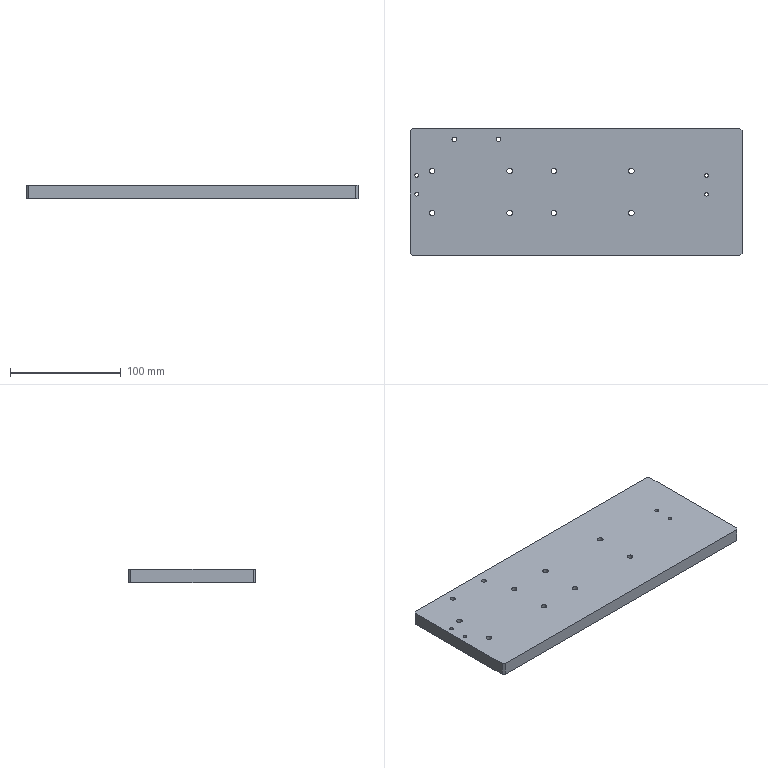Part | SolidWorks | features HoleWzd 3, Chamfer 1, Extrusion 1 | 1 solid | 38 faces | box 300 x 115 x 12 mm | volume 411276 mm3 | cylinder 28 | plane 10 | commonest cylinder face diameters 5 x16 3.3 x8 4.2 x4
STEP:
#1=CARTESIAN_POINT('',(-107.9,47.5,12.));
#2=VERTEX_POINT('',#1);
#3=CARTESIAN_POINT('',(-112.1,47.5,12.));
#4=VERTEX_POINT('',#3);
#5=CARTESIAN_POINT('',(-110.,47.5,12.));
#6=DIRECTION('',(0.,0.,-1.));
#7=DIRECTION('',(-1.,0.,0.));
#8=AXIS2_PLACEMENT_3D('',#5,#6,#7);
#9=CIRCLE('',#8,2.1);
#10=EDGE_CURVE('',#2,#4,#9,.T.);
#11=ORIENTED_EDGE('',*,*,#10,.F.);
#12=CARTESIAN_POINT('',(-107.9,47.5,0.));
#13=VERTEX_POINT('',#12);
#14=CARTESIAN_POINT('',(-107.9,47.5,0.));
#15=DIRECTION('',(0.,0.,-1.));
#16=VECTOR('',#15,1000.);
#17=LINE('',#14,#16);
#18=EDGE_CURVE('',#2,#13,#17,.T.);
#19=ORIENTED_EDGE('',*,*,#18,.T.);
#20=CARTESIAN_POINT('',(-112.1,47.5,0.));
#21=VERTEX_POINT('',#20);
#22=CARTESIAN_POINT('',(-110.,47.5,0.));
#23=DIRECTION('',(0.,0.,-1.));
#24=DIRECTION('',(-1.,0.,0.));
#25=AXIS2_PLACEMENT_3D('',#22,#23,#24);
#26=CIRCLE('',#25,2.1);
#27=EDGE_CURVE('',#13,#21,#26,.T.);
#28=ORIENTED_EDGE('',*,*,#27,.T.);
#29=CARTESIAN_POINT('',(-112.1,47.5,0.));
#30=DIRECTION('',(0.,0.,-1.));
#31=VECTOR('',#30,1000.);
#32=LINE('',#29,#31);
#33=EDGE_CURVE('',#4,#21,#32,.T.);
#34=ORIENTED_EDGE('',*,*,#33,.F.);
#35=EDGE_LOOP('',(#11,#19,#28,#34));
#36=FACE_OUTER_BOUND('',#35,.T.);
#37=CARTESIAN_POINT('',(-110.,47.5,0.));
#38=DIRECTION('',(0.,0.,-1.));
#39=DIRECTION('',(-1.,0.,0.));
#40=AXIS2_PLACEMENT_3D('',#37,#38,#39);
#41=CYLINDRICAL_SURFACE('',#40,2.1);
#42=ADVANCED_FACE('',(#36),#41,.F.);
#43=CARTESIAN_POINT('',(-67.9,47.5,12.));
#44=VERTEX_POINT('',#43);
#45=CARTESIAN_POINT('',(-72.1,47.5,12.));
#46=VERTEX_POINT('',#45);
#47=CARTESIAN_POINT('',(-70.,47.5,12.));
#48=DIRECTION('',(0.,0.,-1.));
#49=DIRECTION('',(-1.,0.,0.));
#50=AXIS2_PLACEMENT_3D('',#47,#48,#49);
#51=CIRCLE('',#50,2.1);
#52=EDGE_CURVE('',#44,#46,#51,.T.);
#53=ORIENTED_EDGE('',*,*,#52,.F.);
#54=CARTESIAN_POINT('',(-67.9,47.5,0.));
#55=VERTEX_POINT('',#54);
#56=CARTESIAN_POINT('',(-67.9,47.5,0.));
#57=DIRECTION('',(0.,0.,-1.));
#58=VECTOR('',#57,1000.);
#59=LINE('',#56,#58);
#60=EDGE_CURVE('',#44,#55,#59,.T.);
#61=ORIENTED_EDGE('',*,*,#60,.T.);
#62=CARTESIAN_POINT('',(-72.1,47.5,0.));
#63=VERTEX_POINT('',#62);
#64=CARTESIAN_POINT('',(-70.,47.5,0.));
#65=DIRECTION('',(0.,0.,-1.));
#66=DIRECTION('',(-1.,0.,0.));
#67=AXIS2_PLACEMENT_3D('',#64,#65,#66);
#68=CIRCLE('',#67,2.1);
#69=EDGE_CURVE('',#55,#63,#68,.T.);
#70=ORIENTED_EDGE('',*,*,#69,.T.);
#71=CARTESIAN_POINT('',(-72.1,47.5,0.));
#72=DIRECTION('',(0.,0.,-1.));
#73=VECTOR('',#72,1000.);
#74=LINE('',#71,#73);
#75=EDGE_CURVE('',#46,#63,#74,.T.);
#76=ORIENTED_EDGE('',*,*,#75,.F.);
#77=EDGE_LOOP('',(#53,#61,#70,#76));
#78=FACE_OUTER_BOUND('',#77,.T.);
#79=CARTESIAN_POINT('',(-70.,47.5,0.));
#80=DIRECTION('',(0.,0.,-1.));
#81=DIRECTION('',(-1.,0.,0.));
#82=AXIS2_PLACEMENT_3D('',#79,#80,#81);
#83=CYLINDRICAL_SURFACE('',#82,2.1);
#84=ADVANCED_FACE('',(#78),#83,.F.);
#85=CARTESIAN_POINT('',(-145.65,15.,0.));
#86=VERTEX_POINT('',#85);
#87=CARTESIAN_POINT('',(-142.35,15.,0.));
#88=VERTEX_POINT('',#87);
#89=CARTESIAN_POINT('',(-144.,15.,0.));
#90=DIRECTION('',(0.,0.,1.));
#91=DIRECTION('',(1.,0.,0.));
#92=AXIS2_PLACEMENT_3D('',#89,#90,#91);
#93=CIRCLE('',#92,1.65);
#94=EDGE_CURVE('',#86,#88,#93,.T.);
#95=ORIENTED_EDGE('',*,*,#94,.F.);
#96=CARTESIAN_POINT('',(-145.65,15.,12.));
#97=VERTEX_POINT('',#96);
#98=CARTESIAN_POINT('',(-145.65,15.,12.));
#99=DIRECTION('',(0.,0.,1.));
#100=VECTOR('',#99,1000.);
#101=LINE('',#98,#100);
#102=EDGE_CURVE('',#86,#97,#101,.T.);
#103=ORIENTED_EDGE('',*,*,#102,.T.);
#104=CARTESIAN_POINT('',(-142.35,15.,12.));
#105=VERTEX_POINT('',#104);
#106=CARTESIAN_POINT('',(-144.,15.,12.));
#107=DIRECTION('',(0.,0.,1.));
#108=DIRECTION('',(1.,0.,0.));
#109=AXIS2_PLACEMENT_3D('',#106,#107,#108);
#110=CIRCLE('',#109,1.65);
#111=EDGE_CURVE('',#97,#105,#110,.T.);
#112=ORIENTED_EDGE('',*,*,#111,.T.);
#113=CARTESIAN_POINT('',(-142.35,15.,12.));
#114=DIRECTION('',(0.,0.,1.));
#115=VECTOR('',#114,1000.);
#116=LINE('',#113,#115);
#117=EDGE_CURVE('',#88,#105,#116,.T.);
#118=ORIENTED_EDGE('',*,*,#117,.F.);
#119=EDGE_LOOP('',(#95,#103,#112,#118));
#120=FACE_OUTER_BOUND('',#119,.T.);
#121=CARTESIAN_POINT('',(-144.,15.,12.));
#122=DIRECTION('',(0.,0.,1.));
#123=DIRECTION('',(1.,0.,0.));
#124=AXIS2_PLACEMENT_3D('',#121,#122,#123);
#125=CYLINDRICAL_SURFACE('',#124,1.65);
#126=ADVANCED_FACE('',(#120),#125,.F.);
#127=CARTESIAN_POINT('',(-145.65,-2.,0.));
#128=VERTEX_POINT('',#127);
#129=CARTESIAN_POINT('',(-142.35,-2.,0.));
#130=VERTEX_POINT('',#129);
#131=CARTESIAN_POINT('',(-144.,-2.,0.));
#132=DIRECTION('',(0.,0.,1.));
#133=DIRECTION('',(1.,0.,0.));
#134=AXIS2_PLACEMENT_3D('',#131,#132,#133);
#135=CIRCLE('',#134,1.65);
#136=EDGE_CURVE('',#128,#130,#135,.T.);
#137=ORIENTED_EDGE('',*,*,#136,.F.);
#138=CARTESIAN_POINT('',(-145.65,-2.,12.));
#139=VERTEX_POINT('',#138);
#140=CARTESIAN_POINT('',(-145.65,-2.,12.));
#141=DIRECTION('',(0.,0.,1.));
#142=VECTOR('',#141,1000.);
#143=LINE('',#140,#142);
#144=EDGE_CURVE('',#128,#139,#143,.T.);
#145=ORIENTED_EDGE('',*,*,#144,.T.);
#146=CARTESIAN_POINT('',(-142.35,-2.,12.));
#147=VERTEX_POINT('',#146);
#148=CARTESIAN_POINT('',(-144.,-2.,12.));
#149=DIRECTION('',(0.,0.,1.));
#150=DIRECTION('',(1.,0.,0.));
#151=AXIS2_PLACEMENT_3D('',#148,#149,#150);
#152=CIRCLE('',#151,1.65);
#153=EDGE_CURVE('',#139,#147,#152,.T.);
#154=ORIENTED_EDGE('',*,*,#153,.T.);
#155=CARTESIAN_POINT('',(-142.35,-2.,12.));
#156=DIRECTION('',(0.,0.,1.));
#157=VECTOR('',#156,1000.);
#158=LINE('',#155,#157);
#159=EDGE_CURVE('',#130,#147,#158,.T.);
#160=ORIENTED_EDGE('',*,*,#159,.F.);
#161=EDGE_LOOP('',(#137,#145,#154,#160));
#162=FACE_OUTER_BOUND('',#161,.T.);
#163=CARTESIAN_POINT('',(-144.,-2.,12.));
#164=DIRECTION('',(0.,0.,1.));
#165=DIRECTION('',(1.,0.,0.));
#166=AXIS2_PLACEMENT_3D('',#163,#164,#165);
#167=CYLINDRICAL_SURFACE('',#166,1.65);
#168=ADVANCED_FACE('',(#162),#167,.F.);
#169=CARTESIAN_POINT('',(116.35,15.,0.));
#170=VERTEX_POINT('',#169);
#171=CARTESIAN_POINT('',(119.65,15.,0.));
#172=VERTEX_POINT('',#171);
#173=CARTESIAN_POINT('',(118.,15.,0.));
#174=DIRECTION('',(0.,0.,1.));
#175=DIRECTION('',(1.,0.,0.));
#176=AXIS2_PLACEMENT_3D('',#173,#174,#175);
#177=CIRCLE('',#176,1.65);
#178=EDGE_CURVE('',#170,#172,#177,.T.);
#179=ORIENTED_EDGE('',*,*,#178,.F.);
#180=CARTESIAN_POINT('',(116.35,15.,12.));
#181=VERTEX_POINT('',#180);
#182=CARTESIAN_POINT('',(116.35,15.,12.));
#183=DIRECTION('',(0.,0.,1.));
#184=VECTOR('',#183,1000.);
#185=LINE('',#182,#184);
#186=EDGE_CURVE('',#170,#181,#185,.T.);
#187=ORIENTED_EDGE('',*,*,#186,.T.);
#188=CARTESIAN_POINT('',(119.65,15.,12.));
#189=VERTEX_POINT('',#188);
#190=CARTESIAN_POINT('',(118.,15.,12.));
#191=DIRECTION('',(0.,0.,1.));
#192=DIRECTION('',(1.,0.,0.));
#193=AXIS2_PLACEMENT_3D('',#190,#191,#192);
#194=CIRCLE('',#193,1.65);
#195=EDGE_CURVE('',#181,#189,#194,.T.);
#196=ORIENTED_EDGE('',*,*,#195,.T.);
#197=CARTESIAN_POINT('',(119.65,15.,12.));
#198=DIRECTION('',(0.,0.,1.));
#199=VECTOR('',#198,1000.);
#200=LINE('',#197,#199);
#201=EDGE_CURVE('',#172,#189,#200,.T.);
#202=ORIENTED_EDGE('',*,*,#201,.F.);
#203=EDGE_LOOP('',(#179,#187,#196,#202));
#204=FACE_OUTER_BOUND('',#203,.T.);
#205=CARTESIAN_POINT('',(118.,15.,12.));
#206=DIRECTION('',(0.,0.,1.));
#207=DIRECTION('',(1.,0.,0.));
#208=AXIS2_PLACEMENT_3D('',#205,#206,#207);
#209=CYLINDRICAL_SURFACE('',#208,1.65);
#210=ADVANCED_FACE('',(#204),#209,.F.);
#211=CARTESIAN_POINT('',(116.35,-2.,0.));
#212=VERTEX_POINT('',#211);
#213=CARTESIAN_POINT('',(119.65,-2.,0.));
#214=VERTEX_POINT('',#213);
#215=CARTESIAN_POINT('',(118.,-2.,0.));
#216=DIRECTION('',(0.,0.,1.));
#217=DIRECTION('',(1.,0.,0.));
#218=AXIS2_PLACEMENT_3D('',#215,#216,#217);
#219=CIRCLE('',#218,1.65);
#220=EDGE_CURVE('',#212,#214,#219,.T.);
#221=ORIENTED_EDGE('',*,*,#220,.F.);
#222=CARTESIAN_POINT('',(116.35,-2.,12.));
#223=VERTEX_POINT('',#222);
#224=CARTESIAN_POINT('',(116.35,-2.,12.));
#225=DIRECTION('',(0.,0.,1.));
#226=VECTOR('',#225,1000.);
#227=LINE('',#224,#226);
#228=EDGE_CURVE('',#212,#223,#227,.T.);
#229=ORIENTED_EDGE('',*,*,#228,.T.);
#230=CARTESIAN_POINT('',(119.65,-2.,12.));
#231=VERTEX_POINT('',#230);
#232=CARTESIAN_POINT('',(118.,-2.,12.));
#233=DIRECTION('',(0.,0.,1.));
#234=DIRECTION('',(1.,0.,0.));
#235=AXIS2_PLACEMENT_3D('',#232,#233,#234);
#236=CIRCLE('',#235,1.65);
#237=EDGE_CURVE('',#223,#231,#236,.T.);
#238=ORIENTED_EDGE('',*,*,#237,.T.);
#239=CARTESIAN_POINT('',(119.65,-2.,12.));
#240=DIRECTION('',(0.,0.,1.));
#241=VECTOR('',#240,1000.);
#242=LINE('',#239,#241);
#243=EDGE_CURVE('',#214,#231,#242,.T.);
#244=ORIENTED_EDGE('',*,*,#243,.F.);
#245=EDGE_LOOP('',(#221,#229,#238,#244));
#246=FACE_OUTER_BOUND('',#245,.T.);
#247=CARTESIAN_POINT('',(118.,-2.,12.));
#248=DIRECTION('',(0.,0.,1.));
#249=DIRECTION('',(1.,0.,0.));
#250=AXIS2_PLACEMENT_3D('',#247,#248,#249);
#251=CYLINDRICAL_SURFACE('',#250,1.65);
#252=ADVANCED_FACE('',(#246),#251,.F.);
#253=CARTESIAN_POINT('',(-127.5,19.,12.));
#254=VERTEX_POINT('',#253);
#255=CARTESIAN_POINT('',(-132.5,19.,12.));
#256=VERTEX_POINT('',#255);
#257=CARTESIAN_POINT('',(-130.,19.,12.));
#258=DIRECTION('',(0.,0.,-1.));
#259=DIRECTION('',(-1.,0.,0.));
#260=AXIS2_PLACEMENT_3D('',#257,#258,#259);
#261=CIRCLE('',#260,2.5);
#262=EDGE_CURVE('',#254,#256,#261,.T.);
#263=ORIENTED_EDGE('',*,*,#262,.F.);
#264=CARTESIAN_POINT('',(-127.5,19.,0.));
#265=VERTEX_POINT('',#264);
#266=CARTESIAN_POINT('',(-127.5,19.,0.));
#267=DIRECTION('',(0.,0.,-1.));
#268=VECTOR('',#267,1000.);
#269=LINE('',#266,#268);
#270=EDGE_CURVE('',#254,#265,#269,.T.);
#271=ORIENTED_EDGE('',*,*,#270,.T.);
#272=CARTESIAN_POINT('',(-132.5,19.,0.));
#273=VERTEX_POINT('',#272);
#274=CARTESIAN_POINT('',(-130.,19.,0.));
#275=DIRECTION('',(0.,0.,-1.));
#276=DIRECTION('',(-1.,0.,0.));
#277=AXIS2_PLACEMENT_3D('',#274,#275,#276);
#278=CIRCLE('',#277,2.5);
#279=EDGE_CURVE('',#265,#273,#278,.T.);
#280=ORIENTED_EDGE('',*,*,#279,.T.);
#281=CARTESIAN_POINT('',(-132.5,19.,0.));
#282=DIRECTION('',(0.,0.,-1.));
#283=VECTOR('',#282,1000.);
#284=LINE('',#281,#283);
#285=EDGE_CURVE('',#256,#273,#284,.T.);
#286=ORIENTED_EDGE('',*,*,#285,.F.);
#287=EDGE_LOOP('',(#263,#271,#280,#286));
#288=FACE_OUTER_BOUND('',#287,.T.);
#289=CARTESIAN_POINT('',(-130.,19.,0.));
#290=DIRECTION('',(0.,0.,-1.));
#291=DIRECTION('',(-1.,0.,0.));
#292=AXIS2_PLACEMENT_3D('',#289,#290,#291);
#293=CYLINDRICAL_SURFACE('',#292,2.5);
#294=ADVANCED_FACE('',(#288),#293,.F.);
#295=CARTESIAN_POINT('',(-57.5,-19.,12.));
#296=VERTEX_POINT('',#295);
#297=CARTESIAN_POINT('',(-62.5,-19.,12.));
#298=VERTEX_POINT('',#297);
#299=CARTESIAN_POINT('',(-60.,-19.,12.));
#300=DIRECTION('',(0.,0.,-1.));
#301=DIRECTION('',(-1.,0.,0.));
#302=AXIS2_PLACEMENT_3D('',#299,#300,#301);
#303=CIRCLE('',#302,2.5);
#304=EDGE_CURVE('',#296,#298,#303,.T.);
#305=ORIENTED_EDGE('',*,*,#304,.F.);
#306=CARTESIAN_POINT('',(-57.5,-19.,0.));
#307=VERTEX_POINT('',#306);
#308=CARTESIAN_POINT('',(-57.5,-19.,0.));
#309=DIRECTION('',(0.,0.,-1.));
#310=VECTOR('',#309,1000.);
#311=LINE('',#308,#310);
#312=EDGE_CURVE('',#296,#307,#311,.T.);
#313=ORIENTED_EDGE('',*,*,#312,.T.);
#314=CARTESIAN_POINT('',(-62.5,-19.,0.));
#315=VERTEX_POINT('',#314);
#316=CARTESIAN_POINT('',(-60.,-19.,0.));
#317=DIRECTION('',(0.,0.,-1.));
#318=DIRECTION('',(-1.,0.,0.));
#319=AXIS2_PLACEMENT_3D('',#316,#317,#318);
#320=CIRCLE('',#319,2.5);
#321=EDGE_CURVE('',#307,#315,#320,.T.);
#322=ORIENTED_EDGE('',*,*,#321,.T.);
#323=CARTESIAN_POINT('',(-62.5,-19.,0.));
#324=DIRECTION('',(0.,0.,-1.));
#325=VECTOR('',#324,1000.);
#326=LINE('',#323,#325);
#327=EDGE_CURVE('',#298,#315,#326,.T.);
#328=ORIENTED_EDGE('',*,*,#327,.F.);
#329=EDGE_LOOP('',(#305,#313,#322,#328));
#330=FACE_OUTER_BOUND('',#329,.T.);
#331=CARTESIAN_POINT('',(-60.,-19.,0.));
#332=DIRECTION('',(0.,0.,-1.));
#333=DIRECTION('',(-1.,0.,0.));
#334=AXIS2_PLACEMENT_3D('',#331,#332,#333);
#335=CYLINDRICAL_SURFACE('',#334,2.5);
#336=ADVANCED_FACE('',(#330),#335,.F.);
#337=CARTESIAN_POINT('',(-57.5,19.,12.));
#338=VERTEX_POINT('',#337);
#339=CARTESIAN_POINT('',(-62.5,19.,12.));
#340=VERTEX_POINT('',#339);
#341=CARTESIAN_POINT('',(-60.,19.,12.));
#342=DIRECTION('',(0.,0.,-1.));
#343=DIRECTION('',(-1.,0.,0.));
#344=AXIS2_PLACEMENT_3D('',#341,#342,#343);
#345=CIRCLE('',#344,2.5);
#346=EDGE_CURVE('',#338,#340,#345,.T.);
#347=ORIENTED_EDGE('',*,*,#346,.F.);
#348=CARTESIAN_POINT('',(-57.5,19.,0.));
#349=VERTEX_POINT('',#348);
#350=CARTESIAN_POINT('',(-57.5,19.,0.));
#351=DIRECTION('',(0.,0.,-1.));
#352=VECTOR('',#351,1000.);
#353=LINE('',#350,#352);
#354=EDGE_CURVE('',#338,#349,#353,.T.);
#355=ORIENTED_EDGE('',*,*,#354,.T.);
#356=CARTESIAN_POINT('',(-62.5,19.,0.));
#357=VERTEX_POINT('',#356);
#358=CARTESIAN_POINT('',(-60.,19.,0.));
#359=DIRECTION('',(0.,0.,-1.));
#360=DIRECTION('',(-1.,0.,0.));
#361=AXIS2_PLACEMENT_3D('',#358,#359,#360);
#362=CIRCLE('',#361,2.5);
#363=EDGE_CURVE('',#349,#357,#362,.T.);
#364=ORIENTED_EDGE('',*,*,#363,.T.);
#365=CARTESIAN_POINT('',(-62.5,19.,0.));
#366=DIRECTION('',(0.,0.,-1.));
#367=VECTOR('',#366,1000.);
#368=LINE('',#365,#367);
#369=EDGE_CURVE('',#340,#357,#368,.T.);
#370=ORIENTED_EDGE('',*,*,#369,.F.);
#371=EDGE_LOOP('',(#347,#355,#364,#370));
#372=FACE_OUTER_BOUND('',#371,.T.);
#373=CARTESIAN_POINT('',(-60.,19.,0.));
#374=DIRECTION('',(0.,0.,-1.));
#375=DIRECTION('',(-1.,0.,0.));
#376=AXIS2_PLACEMENT_3D('',#373,#374,#375);
#377=CYLINDRICAL_SURFACE('',#376,2.5);
#378=ADVANCED_FACE('',(#372),#377,.F.);
#379=CARTESIAN_POINT('',(-127.5,-19.,12.));
#380=VERTEX_POINT('',#379);
#381=CARTESIAN_POINT('',(-132.5,-19.,12.));
#382=VERTEX_POINT('',#381);
#383=CARTESIAN_POINT('',(-130.,-19.,12.));
#384=DIRECTION('',(0.,0.,-1.));
#385=DIRECTION('',(-1.,0.,0.));
#386=AXIS2_PLACEMENT_3D('',#383,#384,#385);
#387=CIRCLE('',#386,2.5);
#388=EDGE_CURVE('',#380,#382,#387,.T.);
#389=ORIENTED_EDGE('',*,*,#388,.F.);
#390=CARTESIAN_POINT('',(-127.5,-19.,0.));
#391=VERTEX_POINT('',#390);
#392=CARTESIAN_POINT('',(-127.5,-19.,0.));
#393=DIRECTION('',(0.,0.,-1.));
#394=VECTOR('',#393,1000.);
#395=LINE('',#392,#394);
#396=EDGE_CURVE('',#380,#391,#395,.T.);
#397=ORIENTED_EDGE('',*,*,#396,.T.);
#398=CARTESIAN_POINT('',(-132.5,-19.,0.));
#399=VERTEX_POINT('',#398);
#400=CARTESIAN_POINT('',(-130.,-19.,0.));
#401=DIRECTION('',(0.,0.,-1.));
#402=DIRECTION('',(-1.,0.,0.));
#403=AXIS2_PLACEMENT_3D('',#400,#401,#402);
#404=CIRCLE('',#403,2.5);
#405=EDGE_CURVE('',#391,#399,#404,.T.);
#406=ORIENTED_EDGE('',*,*,#405,.T.);
#407=CARTESIAN_POINT('',(-132.5,-19.,0.));
#408=DIRECTION('',(0.,0.,-1.));
#409=VECTOR('',#408,1000.);
#410=LINE('',#407,#409);
#411=EDGE_CURVE('',#382,#399,#410,.T.);
#412=ORIENTED_EDGE('',*,*,#411,.F.);
#413=EDGE_LOOP('',(#389,#397,#406,#412));
#414=FACE_OUTER_BOUND('',#413,.T.);
#415=CARTESIAN_POINT('',(-130.,-19.,0.));
#416=DIRECTION('',(0.,0.,-1.));
#417=DIRECTION('',(-1.,0.,0.));
#418=AXIS2_PLACEMENT_3D('',#415,#416,#417);
#419=CYLINDRICAL_SURFACE('',#418,2.5);
#420=ADVANCED_FACE('',(#414),#419,.F.);
#421=CARTESIAN_POINT('',(-17.5,19.,12.));
#422=VERTEX_POINT('',#421);
#423=CARTESIAN_POINT('',(-22.5,19.,12.));
#424=VERTEX_POINT('',#423);
#425=CARTESIAN_POINT('',(-20.,19.,12.));
#426=DIRECTION('',(0.,0.,-1.));
#427=DIRECTION('',(-1.,0.,0.));
#428=AXIS2_PLACEMENT_3D('',#425,#426,#427);
#429=CIRCLE('',#428,2.5);
#430=EDGE_CURVE('',#422,#424,#429,.T.);
#431=ORIENTED_EDGE('',*,*,#430,.F.);
#432=CARTESIAN_POINT('',(-17.5,19.,0.));
#433=VERTEX_POINT('',#432);
#434=CARTESIAN_POINT('',(-17.5,19.,0.));
#435=DIRECTION('',(0.,0.,-1.));
#436=VECTOR('',#435,1000.);
#437=LINE('',#434,#436);
#438=EDGE_CURVE('',#422,#433,#437,.T.);
#439=ORIENTED_EDGE('',*,*,#438,.T.);
#440=CARTESIAN_POINT('',(-22.5,19.,0.));
#441=VERTEX_POINT('',#440);
#442=CARTESIAN_POINT('',(-20.,19.,0.));
#443=DIRECTION('',(0.,0.,-1.));
#444=DIRECTION('',(-1.,0.,0.));
#445=AXIS2_PLACEMENT_3D('',#442,#443,#444);
#446=CIRCLE('',#445,2.5);
#447=EDGE_CURVE('',#433,#441,#446,.T.);
#448=ORIENTED_EDGE('',*,*,#447,.T.);
#449=CARTESIAN_POINT('',(-22.5,19.,0.));
#450=DIRECTION('',(0.,0.,-1.));
#451=VECTOR('',#450,1000.);
#452=LINE('',#449,#451);
#453=EDGE_CURVE('',#424,#441,#452,.T.);
#454=ORIENTED_EDGE('',*,*,#453,.F.);
#455=EDGE_LOOP('',(#431,#439,#448,#454));
#456=FACE_OUTER_BOUND('',#455,.T.);
#457=CARTESIAN_POINT('',(-20.,19.,0.));
#458=DIRECTION('',(0.,0.,-1.));
#459=DIRECTION('',(-1.,0.,0.));
#460=AXIS2_PLACEMENT_3D('',#457,#458,#459);
#461=CYLINDRICAL_SURFACE('',#460,2.5);
#462=ADVANCED_FACE('',(#456),#461,.F.);
#463=CARTESIAN_POINT('',(52.5,-19.,12.));
#464=VERTEX_POINT('',#463);
#465=CARTESIAN_POINT('',(47.5,-19.,12.));
#466=VERTEX_POINT('',#465);
#467=CARTESIAN_POINT('',(50.,-19.,12.));
#468=DIRECTION('',(0.,0.,-1.));
#469=DIRECTION('',(-1.,0.,0.));
#470=AXIS2_PLACEMENT_3D('',#467,#468,#469);
#471=CIRCLE('',#470,2.5);
#472=EDGE_CURVE('',#464,#466,#471,.T.);
#473=ORIENTED_EDGE('',*,*,#472,.F.);
#474=CARTESIAN_POINT('',(52.5,-19.,0.));
#475=VERTEX_POINT('',#474);
#476=CARTESIAN_POINT('',(52.5,-19.,0.));
#477=DIRECTION('',(0.,0.,-1.));
#478=VECTOR('',#477,1000.);
#479=LINE('',#476,#478);
#480=EDGE_CURVE('',#464,#475,#479,.T.);
#481=ORIENTED_EDGE('',*,*,#480,.T.);
#482=CARTESIAN_POINT('',(47.5,-19.,0.));
#483=VERTEX_POINT('',#482);
#484=CARTESIAN_POINT('',(50.,-19.,0.));
#485=DIRECTION('',(0.,0.,-1.));
#486=DIRECTION('',(-1.,0.,0.));
#487=AXIS2_PLACEMENT_3D('',#484,#485,#486);
#488=CIRCLE('',#487,2.5);
#489=EDGE_CURVE('',#475,#483,#488,.T.);
#490=ORIENTED_EDGE('',*,*,#489,.T.);
#491=CARTESIAN_POINT('',(47.5,-19.,0.));
#492=DIRECTION('',(0.,0.,-1.));
#493=VECTOR('',#492,1000.);
#494=LINE('',#491,#493);
#495=EDGE_CURVE('',#466,#483,#494,.T.);
#496=ORIENTED_EDGE('',*,*,#495,.F.);
#497=EDGE_LOOP('',(#473,#481,#490,#496));
#498=FACE_OUTER_BOUND('',#497,.T.);
#499=CARTESIAN_POINT('',(50.,-19.,0.));
#500=DIRECTION('',(0.,0.,-1.));
#501=DIRECTION('',(-1.,0.,0.));
#502=AXIS2_PLACEMENT_3D('',#499,#500,#501);
#503=CYLINDRICAL_SURFACE('',#502,2.5);
#504=ADVANCED_FACE('',(#498),#503,.F.);
#505=CARTESIAN_POINT('',(52.5,19.,12.));
#506=VERTEX_POINT('',#505);
#507=CARTESIAN_POINT('',(47.5,19.,12.));
#508=VERTEX_POINT('',#507);
#509=CARTESIAN_POINT('',(50.,19.,12.));
#510=DIRECTION('',(0.,0.,-1.));
#511=DIRECTION('',(-1.,0.,0.));
#512=AXIS2_PLACEMENT_3D('',#509,#510,#511);
#513=CIRCLE('',#512,2.5);
#514=EDGE_CURVE('',#506,#508,#513,.T.);
#515=ORIENTED_EDGE('',*,*,#514,.F.);
#516=CARTESIAN_POINT('',(52.5,19.,0.));
#517=VERTEX_POINT('',#516);
#518=CARTESIAN_POINT('',(52.5,19.,0.));
#519=DIRECTION('',(0.,0.,-1.));
#520=VECTOR('',#519,1000.);
#521=LINE('',#518,#520);
#522=EDGE_CURVE('',#506,#517,#521,.T.);
#523=ORIENTED_EDGE('',*,*,#522,.T.);
#524=CARTESIAN_POINT('',(47.5,19.,0.));
#525=VERTEX_POINT('',#524);
#526=CARTESIAN_POINT('',(50.,19.,0.));
#527=DIRECTION('',(0.,0.,-1.));
#528=DIRECTION('',(-1.,0.,0.));
#529=AXIS2_PLACEMENT_3D('',#526,#527,#528);
#530=CIRCLE('',#529,2.5);
#531=EDGE_CURVE('',#517,#525,#530,.T.);
#532=ORIENTED_EDGE('',*,*,#531,.T.);
#533=CARTESIAN_POINT('',(47.5,19.,0.));
#534=DIRECTION('',(0.,0.,-1.));
#535=VECTOR('',#534,1000.);
#536=LINE('',#533,#535);
#537=EDGE_CURVE('',#508,#525,#536,.T.);
#538=ORIENTED_EDGE('',*,*,#537,.F.);
#539=EDGE_LOOP('',(#515,#523,#532,#538));
#540=FACE_OUTER_BOUND('',#539,.T.);
#541=CARTESIAN_POINT('',(50.,19.,0.));
#542=DIRECTION('',(0.,0.,-1.));
#543=DIRECTION('',(-1.,0.,0.));
#544=AXIS2_PLACEMENT_3D('',#541,#542,#543);
#545=CYLINDRICAL_SURFACE('',#544,2.5);
#546=ADVANCED_FACE('',(#540),#545,.F.);
#547=CARTESIAN_POINT('',(-17.5,-19.,12.));
#548=VERTEX_POINT('',#547);
#549=CARTESIAN_POINT('',(-22.5,-19.,12.));
#550=VERTEX_POINT('',#549);
#551=CARTESIAN_POINT('',(-20.,-19.,12.));
#552=DIRECTION('',(0.,0.,-1.));
#553=DIRECTION('',(-1.,0.,0.));
#554=AXIS2_PLACEMENT_3D('',#551,#552,#553);
#555=CIRCLE('',#554,2.5);
#556=EDGE_CURVE('',#548,#550,#555,.T.);
#557=ORIENTED_EDGE('',*,*,#556,.F.);
#558=CARTESIAN_POINT('',(-17.5,-19.,0.));
#559=VERTEX_POINT('',#558);
#560=CARTESIAN_POINT('',(-17.5,-19.,0.));
#561=DIRECTION('',(0.,0.,-1.));
#562=VECTOR('',#561,1000.);
#563=LINE('',#560,#562);
#564=EDGE_CURVE('',#548,#559,#563,.T.);
#565=ORIENTED_EDGE('',*,*,#564,.T.);
#566=CARTESIAN_POINT('',(-22.5,-19.,0.));
#567=VERTEX_POINT('',#566);
#568=CARTESIAN_POINT('',(-20.,-19.,0.));
#569=DIRECTION('',(0.,0.,-1.));
#570=DIRECTION('',(-1.,0.,0.));
#571=AXIS2_PLACEMENT_3D('',#568,#569,#570);
#572=CIRCLE('',#571,2.5);
#573=EDGE_CURVE('',#559,#567,#572,.T.);
#574=ORIENTED_EDGE('',*,*,#573,.T.);
#575=CARTESIAN_POINT('',(-22.5,-19.,0.));
#576=DIRECTION('',(0.,0.,-1.));
#577=VECTOR('',#576,1000.);
#578=LINE('',#575,#577);
#579=EDGE_CURVE('',#550,#567,#578,.T.);
#580=ORIENTED_EDGE('',*,*,#579,.F.);
#581=EDGE_LOOP('',(#557,#565,#574,#580));
#582=FACE_OUTER_BOUND('',#581,.T.);
#583=CARTESIAN_POINT('',(-20.,-19.,0.));
#584=DIRECTION('',(0.,0.,-1.));
#585=DIRECTION('',(-1.,0.,0.));
#586=AXIS2_PLACEMENT_3D('',#583,#584,#585);
#587=CYLINDRICAL_SURFACE('',#586,2.5);
#588=ADVANCED_FACE('',(#582),#587,.F.);
#589=CARTESIAN_POINT('',(150.,-55.5,0.));
#590=VERTEX_POINT('',#589);
#591=CARTESIAN_POINT('',(150.,55.5,0.));
#592=VERTEX_POINT('',#591);
#593=CARTESIAN_POINT('',(150.,-57.5,0.));
#594=DIRECTION('',(0.,1.,0.));
#595=VECTOR('',#594,1000.);
#596=LINE('',#593,#595);
#597=EDGE_CURVE('',#590,#592,#596,.T.);
#598=ORIENTED_EDGE('',*,*,#597,.T.);
#599=CARTESIAN_POINT('',(150.,55.5,12.));
#600=VERTEX_POINT('',#599);
#601=CARTESIAN_POINT('',(150.,55.5,12.));
#602=DIRECTION('',(0.,0.,1.));
#603=VECTOR('',#602,1000.);
#604=LINE('',#601,#603);
#605=EDGE_CURVE('',#592,#600,#604,.T.);
#606=ORIENTED_EDGE('',*,*,#605,.T.);
#607=CARTESIAN_POINT('',(150.,-55.5,12.));
#608=VERTEX_POINT('',#607);
#609=CARTESIAN_POINT('',(150.,-57.5,12.));
#610=DIRECTION('',(0.,1.,0.));
#611=VECTOR('',#610,1000.);
#612=LINE('',#609,#611);
#613=EDGE_CURVE('',#608,#600,#612,.T.);
#614=ORIENTED_EDGE('',*,*,#613,.F.);
#615=CARTESIAN_POINT('',(150.,-55.5,12.));
#616=DIRECTION('',(0.,0.,-1.));
#617=VECTOR('',#616,1000.);
#618=LINE('',#615,#617);
#619=EDGE_CURVE('',#608,#590,#618,.T.);
#620=ORIENTED_EDGE('',*,*,#619,.T.);
#621=EDGE_LOOP('',(#598,#606,#614,#620));
#622=FACE_OUTER_BOUND('',#621,.T.);
#623=CARTESIAN_POINT('',(150.,-57.5,12.));
#624=DIRECTION('',(-1.,0.,0.));
#625=DIRECTION('',(0.,0.,1.));
#626=AXIS2_PLACEMENT_3D('',#623,#624,#625);
#627=PLANE('',#626);
#628=ADVANCED_FACE('',(#622),#627,.F.);
#629=CARTESIAN_POINT('',(148.,57.5,12.));
#630=VERTEX_POINT('',#629);
#631=CARTESIAN_POINT('',(-148.,57.5,12.));
#632=VERTEX_POINT('',#631);
#633=CARTESIAN_POINT('',(-150.,57.5,12.));
#634=DIRECTION('',(-1.,0.,0.));
#635=VECTOR('',#634,1000.);
#636=LINE('',#633,#635);
#637=EDGE_CURVE('',#630,#632,#636,.T.);
#638=ORIENTED_EDGE('',*,*,#637,.F.);
#639=CARTESIAN_POINT('',(148.,57.5,0.));
#640=VERTEX_POINT('',#639);
#641=CARTESIAN_POINT('',(148.,57.5,12.));
#642=DIRECTION('',(0.,0.,-1.));
#643=VECTOR('',#642,1000.);
#644=LINE('',#641,#643);
#645=EDGE_CURVE('',#630,#640,#644,.T.);
#646=ORIENTED_EDGE('',*,*,#645,.T.);
#647=CARTESIAN_POINT('',(-148.,57.5,0.));
#648=VERTEX_POINT('',#647);
#649=CARTESIAN_POINT('',(-150.,57.5,0.));
#650=DIRECTION('',(-1.,0.,0.));
#651=VECTOR('',#650,1000.);
#652=LINE('',#649,#651);
#653=EDGE_CURVE('',#640,#648,#652,.T.);
#654=ORIENTED_EDGE('',*,*,#653,.T.);
#655=CARTESIAN_POINT('',(-148.,57.5,12.));
#656=DIRECTION('',(0.,0.,1.));
#657=VECTOR('',#656,1000.);
#658=LINE('',#655,#657);
#659=EDGE_CURVE('',#648,#632,#658,.T.);
#660=ORIENTED_EDGE('',*,*,#659,.T.);
#661=EDGE_LOOP('',(#638,#646,#654,#660));
#662=FACE_OUTER_BOUND('',#661,.T.);
#663=CARTESIAN_POINT('',(-150.,57.5,12.));
#664=DIRECTION('',(0.,-1.,0.));
#665=DIRECTION('',(0.,0.,-1.));
#666=AXIS2_PLACEMENT_3D('',#663,#664,#665);
#667=PLANE('',#666);
#668=ADVANCED_FACE('',(#662),#667,.F.);
#669=CARTESIAN_POINT('',(-150.,55.5,12.));
#670=VERTEX_POINT('',#669);
#671=CARTESIAN_POINT('',(-150.,-55.5,12.));
#672=VERTEX_POINT('',#671);
#673=CARTESIAN_POINT('',(-150.,-57.5,12.));
#674=DIRECTION('',(0.,-1.,0.));
#675=VECTOR('',#674,1000.);
#676=LINE('',#673,#675);
#677=EDGE_CURVE('',#670,#672,#676,.T.);
#678=ORIENTED_EDGE('',*,*,#677,.F.);
#679=CARTESIAN_POINT('',(-150.,55.5,0.));
#680=VERTEX_POINT('',#679);
#681=CARTESIAN_POINT('',(-150.,55.5,12.));
#682=DIRECTION('',(0.,0.,-1.));
#683=VECTOR('',#682,1000.);
#684=LINE('',#681,#683);
#685=EDGE_CURVE('',#670,#680,#684,.T.);
#686=ORIENTED_EDGE('',*,*,#685,.T.);
#687=CARTESIAN_POINT('',(-150.,-55.5,0.));
#688=VERTEX_POINT('',#687);
#689=CARTESIAN_POINT('',(-150.,-57.5,0.));
#690=DIRECTION('',(0.,-1.,0.));
#691=VECTOR('',#690,1000.);
#692=LINE('',#689,#691);
#693=EDGE_CURVE('',#680,#688,#692,.T.);
#694=ORIENTED_EDGE('',*,*,#693,.T.);
#695=CARTESIAN_POINT('',(-150.,-55.5,12.));
#696=DIRECTION('',(0.,0.,1.));
#697=VECTOR('',#696,1000.);
#698=LINE('',#695,#697);
#699=EDGE_CURVE('',#688,#672,#698,.T.);
#700=ORIENTED_EDGE('',*,*,#699,.T.);
#701=EDGE_LOOP('',(#678,#686,#694,#700));
#702=FACE_OUTER_BOUND('',#701,.T.);
#703=CARTESIAN_POINT('',(-150.,-57.5,12.));
#704=DIRECTION('',(1.,0.,0.));
#705=DIRECTION('',(0.,0.,-1.));
#706=AXIS2_PLACEMENT_3D('',#703,#704,#705);
#707=PLANE('',#706);
#708=ADVANCED_FACE('',(#702),#707,.F.);
#709=CARTESIAN_POINT('',(-148.,-57.5,0.));
#710=VERTEX_POINT('',#709);
#711=CARTESIAN_POINT('',(148.,-57.5,0.));
#712=VERTEX_POINT('',#711);
#713=CARTESIAN_POINT('',(-150.,-57.5,0.));
#714=DIRECTION('',(1.,0.,0.));
#715=VECTOR('',#714,1000.);
#716=LINE('',#713,#715);
#717=EDGE_CURVE('',#710,#712,#716,.T.);
#718=ORIENTED_EDGE('',*,*,#717,.T.);
#719=CARTESIAN_POINT('',(148.,-57.5,12.));
#720=VERTEX_POINT('',#719);
#721=CARTESIAN_POINT('',(148.,-57.5,12.));
#722=DIRECTION('',(0.,0.,1.));
#723=VECTOR('',#722,1000.);
#724=LINE('',#721,#723);
#725=EDGE_CURVE('',#712,#720,#724,.T.);
#726=ORIENTED_EDGE('',*,*,#725,.T.);
#727=CARTESIAN_POINT('',(-148.,-57.5,12.));
#728=VERTEX_POINT('',#727);
#729=CARTESIAN_POINT('',(-150.,-57.5,12.));
#730=DIRECTION('',(1.,0.,0.));
#731=VECTOR('',#730,1000.);
#732=LINE('',#729,#731);
#733=EDGE_CURVE('',#728,#720,#732,.T.);
#734=ORIENTED_EDGE('',*,*,#733,.F.);
#735=CARTESIAN_POINT('',(-148.,-57.5,12.));
#736=DIRECTION('',(0.,0.,-1.));
#737=VECTOR('',#736,1000.);
#738=LINE('',#735,#737);
#739=EDGE_CURVE('',#728,#710,#738,.T.);
#740=ORIENTED_EDGE('',*,*,#739,.T.);
#741=EDGE_LOOP('',(#718,#726,#734,#740));
#742=FACE_OUTER_BOUND('',#741,.T.);
#743=CARTESIAN_POINT('',(-150.,-57.5,12.));
#744=DIRECTION('',(0.,1.,0.));
#745=DIRECTION('',(0.,0.,1.));
#746=AXIS2_PLACEMENT_3D('',#743,#744,#745);
#747=PLANE('',#746);
#748=ADVANCED_FACE('',(#742),#747,.F.);
#749=CARTESIAN_POINT('',(-110.,47.5,12.));
#750=DIRECTION('',(0.,0.,-1.));
#751=DIRECTION('',(-1.,0.,0.));
#752=AXIS2_PLACEMENT_3D('',#749,#750,#751);
#753=CIRCLE('',#752,2.1);
#754=EDGE_CURVE('',#4,#2,#753,.T.);
#755=ORIENTED_EDGE('',*,*,#754,.T.);
#756=ORIENTED_EDGE('',*,*,#10,.T.);
#757=EDGE_LOOP('',(#755,#756));
#758=FACE_BOUND('',#757,.T.);
#759=CARTESIAN_POINT('',(-70.,47.5,12.));
#760=DIRECTION('',(0.,0.,-1.));
#761=DIRECTION('',(-1.,0.,0.));
#762=AXIS2_PLACEMENT_3D('',#759,#760,#761);
#763=CIRCLE('',#762,2.1);
#764=EDGE_CURVE('',#46,#44,#763,.T.);
#765=ORIENTED_EDGE('',*,*,#764,.T.);
#766=ORIENTED_EDGE('',*,*,#52,.T.);
#767=EDGE_LOOP('',(#765,#766));
#768=FACE_BOUND('',#767,.T.);
#769=CARTESIAN_POINT('',(-144.,15.,12.));
#770=DIRECTION('',(0.,0.,1.));
#771=DIRECTION('',(1.,0.,0.));
#772=AXIS2_PLACEMENT_3D('',#769,#770,#771);
#773=CIRCLE('',#772,1.65);
#774=EDGE_CURVE('',#105,#97,#773,.T.);
#775=ORIENTED_EDGE('',*,*,#774,.F.);
#776=ORIENTED_EDGE('',*,*,#111,.F.);
#777=EDGE_LOOP('',(#775,#776));
#778=FACE_BOUND('',#777,.T.);
#779=CARTESIAN_POINT('',(-144.,-2.,12.));
#780=DIRECTION('',(0.,0.,1.));
#781=DIRECTION('',(1.,0.,0.));
#782=AXIS2_PLACEMENT_3D('',#779,#780,#781);
#783=CIRCLE('',#782,1.65);
#784=EDGE_CURVE('',#147,#139,#783,.T.);
#785=ORIENTED_EDGE('',*,*,#784,.F.);
#786=ORIENTED_EDGE('',*,*,#153,.F.);
#787=EDGE_LOOP('',(#785,#786));
#788=FACE_BOUND('',#787,.T.);
#789=CARTESIAN_POINT('',(118.,15.,12.));
#790=DIRECTION('',(0.,0.,1.));
#791=DIRECTION('',(1.,0.,0.));
#792=AXIS2_PLACEMENT_3D('',#789,#790,#791);
#793=CIRCLE('',#792,1.65);
#794=EDGE_CURVE('',#189,#181,#793,.T.);
#795=ORIENTED_EDGE('',*,*,#794,.F.);
#796=ORIENTED_EDGE('',*,*,#195,.F.);
#797=EDGE_LOOP('',(#795,#796));
#798=FACE_BOUND('',#797,.T.);
#799=CARTESIAN_POINT('',(118.,-2.,12.));
#800=DIRECTION('',(0.,0.,1.));
#801=DIRECTION('',(1.,0.,0.));
#802=AXIS2_PLACEMENT_3D('',#799,#800,#801);
#803=CIRCLE('',#802,1.65);
#804=EDGE_CURVE('',#231,#223,#803,.T.);
#805=ORIENTED_EDGE('',*,*,#804,.F.);
#806=ORIENTED_EDGE('',*,*,#237,.F.);
#807=EDGE_LOOP('',(#805,#806));
#808=FACE_BOUND('',#807,.T.);
#809=CARTESIAN_POINT('',(-130.,19.,12.));
#810=DIRECTION('',(0.,0.,-1.));
#811=DIRECTION('',(-1.,0.,0.));
#812=AXIS2_PLACEMENT_3D('',#809,#810,#811);
#813=CIRCLE('',#812,2.5);
#814=EDGE_CURVE('',#256,#254,#813,.T.);
#815=ORIENTED_EDGE('',*,*,#814,.T.);
#816=ORIENTED_EDGE('',*,*,#262,.T.);
#817=EDGE_LOOP('',(#815,#816));
#818=FACE_BOUND('',#817,.T.);
#819=CARTESIAN_POINT('',(-60.,-19.,12.));
#820=DIRECTION('',(0.,0.,-1.));
#821=DIRECTION('',(-1.,0.,0.));
#822=AXIS2_PLACEMENT_3D('',#819,#820,#821);
#823=CIRCLE('',#822,2.5);
#824=EDGE_CURVE('',#298,#296,#823,.T.);
#825=ORIENTED_EDGE('',*,*,#824,.T.);
#826=ORIENTED_EDGE('',*,*,#304,.T.);
#827=EDGE_LOOP('',(#825,#826));
#828=FACE_BOUND('',#827,.T.);
#829=CARTESIAN_POINT('',(-60.,19.,12.));
#830=DIRECTION('',(0.,0.,-1.));
#831=DIRECTION('',(-1.,0.,0.));
#832=AXIS2_PLACEMENT_3D('',#829,#830,#831);
#833=CIRCLE('',#832,2.5);
#834=EDGE_CURVE('',#340,#338,#833,.T.);
#835=ORIENTED_EDGE('',*,*,#834,.T.);
#836=ORIENTED_EDGE('',*,*,#346,.T.);
#837=EDGE_LOOP('',(#835,#836));
#838=FACE_BOUND('',#837,.T.);
#839=CARTESIAN_POINT('',(-130.,-19.,12.));
#840=DIRECTION('',(0.,0.,-1.));
#841=DIRECTION('',(-1.,0.,0.));
#842=AXIS2_PLACEMENT_3D('',#839,#840,#841);
#843=CIRCLE('',#842,2.5);
#844=EDGE_CURVE('',#382,#380,#843,.T.);
#845=ORIENTED_EDGE('',*,*,#844,.T.);
#846=ORIENTED_EDGE('',*,*,#388,.T.);
#847=EDGE_LOOP('',(#845,#846));
#848=FACE_BOUND('',#847,.T.);
#849=CARTESIAN_POINT('',(-20.,19.,12.));
#850=DIRECTION('',(0.,0.,-1.));
#851=DIRECTION('',(-1.,0.,0.));
#852=AXIS2_PLACEMENT_3D('',#849,#850,#851);
#853=CIRCLE('',#852,2.5);
#854=EDGE_CURVE('',#424,#422,#853,.T.);
#855=ORIENTED_EDGE('',*,*,#854,.T.);
#856=ORIENTED_EDGE('',*,*,#430,.T.);
#857=EDGE_LOOP('',(#855,#856));
#858=FACE_BOUND('',#857,.T.);
#859=CARTESIAN_POINT('',(50.,-19.,12.));
#860=DIRECTION('',(0.,0.,-1.));
#861=DIRECTION('',(-1.,0.,0.));
#862=AXIS2_PLACEMENT_3D('',#859,#860,#861);
#863=CIRCLE('',#862,2.5);
#864=EDGE_CURVE('',#466,#464,#863,.T.);
#865=ORIENTED_EDGE('',*,*,#864,.T.);
#866=ORIENTED_EDGE('',*,*,#472,.T.);
#867=EDGE_LOOP('',(#865,#866));
#868=FACE_BOUND('',#867,.T.);
#869=CARTESIAN_POINT('',(50.,19.,12.));
#870=DIRECTION('',(0.,0.,-1.));
#871=DIRECTION('',(-1.,0.,0.));
#872=AXIS2_PLACEMENT_3D('',#869,#870,#871);
#873=CIRCLE('',#872,2.5);
#874=EDGE_CURVE('',#508,#506,#873,.T.);
#875=ORIENTED_EDGE('',*,*,#874,.T.);
#876=ORIENTED_EDGE('',*,*,#514,.T.);
#877=EDGE_LOOP('',(#875,#876));
#878=FACE_BOUND('',#877,.T.);
#879=CARTESIAN_POINT('',(-20.,-19.,12.));
#880=DIRECTION('',(0.,0.,-1.));
#881=DIRECTION('',(-1.,0.,0.));
#882=AXIS2_PLACEMENT_3D('',#879,#880,#881);
#883=CIRCLE('',#882,2.5);
#884=EDGE_CURVE('',#550,#548,#883,.T.);
#885=ORIENTED_EDGE('',*,*,#884,.T.);
#886=ORIENTED_EDGE('',*,*,#556,.T.);
#887=EDGE_LOOP('',(#885,#886));
#888=FACE_BOUND('',#887,.T.);
#889=ORIENTED_EDGE('',*,*,#613,.T.);
#890=CARTESIAN_POINT('',(148.,57.5,12.));
#891=DIRECTION('',(-0.7071,0.7071,0.));
#892=VECTOR('',#891,1000.);
#893=LINE('',#890,#892);
#894=EDGE_CURVE('',#600,#630,#893,.T.);
#895=ORIENTED_EDGE('',*,*,#894,.T.);
#896=ORIENTED_EDGE('',*,*,#637,.T.);
#897=CARTESIAN_POINT('',(-150.,55.5,12.));
#898=DIRECTION('',(-0.7071,-0.7071,0.));
#899=VECTOR('',#898,1000.);
#900=LINE('',#897,#899);
#901=EDGE_CURVE('',#632,#670,#900,.T.);
#902=ORIENTED_EDGE('',*,*,#901,.T.);
#903=ORIENTED_EDGE('',*,*,#677,.T.);
#904=CARTESIAN_POINT('',(-148.,-57.5,12.));
#905=DIRECTION('',(0.7071,-0.7071,0.));
#906=VECTOR('',#905,1000.);
#907=LINE('',#904,#906);
#908=EDGE_CURVE('',#672,#728,#907,.T.);
#909=ORIENTED_EDGE('',*,*,#908,.T.);
#910=ORIENTED_EDGE('',*,*,#733,.T.);
#911=CARTESIAN_POINT('',(150.,-55.5,12.));
#912=DIRECTION('',(0.7071,0.7071,0.));
#913=VECTOR('',#912,1000.);
#914=LINE('',#911,#913);
#915=EDGE_CURVE('',#720,#608,#914,.T.);
#916=ORIENTED_EDGE('',*,*,#915,.T.);
#917=EDGE_LOOP('',(#889,#895,#896,#902,#903,#909,#910,#916));
#918=FACE_OUTER_BOUND('',#917,.T.);
#919=CARTESIAN_POINT('',(0.,0.,12.));
#920=DIRECTION('',(0.,0.,-1.));
#921=DIRECTION('',(-1.,0.,0.));
#922=AXIS2_PLACEMENT_3D('',#919,#920,#921);
#923=PLANE('',#922);
#924=ADVANCED_FACE('',(#758,#768,#778,#788,#798,#808,#818,#828,#838,#848,#858,#868,#878,#888,#918),#923,.F.);
#925=CARTESIAN_POINT('',(-110.,47.5,0.));
#926=DIRECTION('',(0.,0.,-1.));
#927=DIRECTION('',(-1.,0.,0.));
#928=AXIS2_PLACEMENT_3D('',#925,#926,#927);
#929=CIRCLE('',#928,2.1);
#930=EDGE_CURVE('',#21,#13,#929,.T.);
#931=ORIENTED_EDGE('',*,*,#930,.F.);
#932=ORIENTED_EDGE('',*,*,#27,.F.);
#933=EDGE_LOOP('',(#931,#932));
#934=FACE_BOUND('',#933,.T.);
#935=CARTESIAN_POINT('',(-70.,47.5,0.));
#936=DIRECTION('',(0.,0.,-1.));
#937=DIRECTION('',(-1.,0.,0.));
#938=AXIS2_PLACEMENT_3D('',#935,#936,#937);
#939=CIRCLE('',#938,2.1);
#940=EDGE_CURVE('',#63,#55,#939,.T.);
#941=ORIENTED_EDGE('',*,*,#940,.F.);
#942=ORIENTED_EDGE('',*,*,#69,.F.);
#943=EDGE_LOOP('',(#941,#942));
#944=FACE_BOUND('',#943,.T.);
#945=CARTESIAN_POINT('',(-144.,15.,0.));
#946=DIRECTION('',(0.,0.,1.));
#947=DIRECTION('',(1.,0.,0.));
#948=AXIS2_PLACEMENT_3D('',#945,#946,#947);
#949=CIRCLE('',#948,1.65);
#950=EDGE_CURVE('',#88,#86,#949,.T.);
#951=ORIENTED_EDGE('',*,*,#950,.T.);
#952=ORIENTED_EDGE('',*,*,#94,.T.);
#953=EDGE_LOOP('',(#951,#952));
#954=FACE_BOUND('',#953,.T.);
#955=CARTESIAN_POINT('',(-144.,-2.,0.));
#956=DIRECTION('',(0.,0.,1.));
#957=DIRECTION('',(1.,0.,0.));
#958=AXIS2_PLACEMENT_3D('',#955,#956,#957);
#959=CIRCLE('',#958,1.65);
#960=EDGE_CURVE('',#130,#128,#959,.T.);
#961=ORIENTED_EDGE('',*,*,#960,.T.);
#962=ORIENTED_EDGE('',*,*,#136,.T.);
#963=EDGE_LOOP('',(#961,#962));
#964=FACE_BOUND('',#963,.T.);
#965=CARTESIAN_POINT('',(118.,15.,0.));
#966=DIRECTION('',(0.,0.,1.));
#967=DIRECTION('',(1.,0.,0.));
#968=AXIS2_PLACEMENT_3D('',#965,#966,#967);
#969=CIRCLE('',#968,1.65);
#970=EDGE_CURVE('',#172,#170,#969,.T.);
#971=ORIENTED_EDGE('',*,*,#970,.T.);
#972=ORIENTED_EDGE('',*,*,#178,.T.);
#973=EDGE_LOOP('',(#971,#972));
#974=FACE_BOUND('',#973,.T.);
#975=CARTESIAN_POINT('',(118.,-2.,0.));
#976=DIRECTION('',(0.,0.,1.));
#977=DIRECTION('',(1.,0.,0.));
#978=AXIS2_PLACEMENT_3D('',#975,#976,#977);
#979=CIRCLE('',#978,1.65);
#980=EDGE_CURVE('',#214,#212,#979,.T.);
#981=ORIENTED_EDGE('',*,*,#980,.T.);
#982=ORIENTED_EDGE('',*,*,#220,.T.);
#983=EDGE_LOOP('',(#981,#982));
#984=FACE_BOUND('',#983,.T.);
#985=CARTESIAN_POINT('',(-130.,19.,0.));
#986=DIRECTION('',(0.,0.,-1.));
#987=DIRECTION('',(-1.,0.,0.));
#988=AXIS2_PLACEMENT_3D('',#985,#986,#987);
#989=CIRCLE('',#988,2.5);
#990=EDGE_CURVE('',#273,#265,#989,.T.);
#991=ORIENTED_EDGE('',*,*,#990,.F.);
#992=ORIENTED_EDGE('',*,*,#279,.F.);
#993=EDGE_LOOP('',(#991,#992));
#994=FACE_BOUND('',#993,.T.);
#995=CARTESIAN_POINT('',(-60.,-19.,0.));
#996=DIRECTION('',(0.,0.,-1.));
#997=DIRECTION('',(-1.,0.,0.));
#998=AXIS2_PLACEMENT_3D('',#995,#996,#997);
#999=CIRCLE('',#998,2.5);
#1000=EDGE_CURVE('',#315,#307,#999,.T.);
#1001=ORIENTED_EDGE('',*,*,#1000,.F.);
#1002=ORIENTED_EDGE('',*,*,#321,.F.);
#1003=EDGE_LOOP('',(#1001,#1002));
#1004=FACE_BOUND('',#1003,.T.);
#1005=CARTESIAN_POINT('',(-60.,19.,0.));
#1006=DIRECTION('',(0.,0.,-1.));
#1007=DIRECTION('',(-1.,0.,0.));
#1008=AXIS2_PLACEMENT_3D('',#1005,#1006,#1007);
#1009=CIRCLE('',#1008,2.5);
#1010=EDGE_CURVE('',#357,#349,#1009,.T.);
#1011=ORIENTED_EDGE('',*,*,#1010,.F.);
#1012=ORIENTED_EDGE('',*,*,#363,.F.);
#1013=EDGE_LOOP('',(#1011,#1012));
#1014=FACE_BOUND('',#1013,.T.);
#1015=CARTESIAN_POINT('',(-130.,-19.,0.));
#1016=DIRECTION('',(0.,0.,-1.));
#1017=DIRECTION('',(-1.,0.,0.));
#1018=AXIS2_PLACEMENT_3D('',#1015,#1016,#1017);
#1019=CIRCLE('',#1018,2.5);
#1020=EDGE_CURVE('',#399,#391,#1019,.T.);
#1021=ORIENTED_EDGE('',*,*,#1020,.F.);
#1022=ORIENTED_EDGE('',*,*,#405,.F.);
#1023=EDGE_LOOP('',(#1021,#1022));
#1024=FACE_BOUND('',#1023,.T.);
#1025=CARTESIAN_POINT('',(-20.,19.,0.));
#1026=DIRECTION('',(0.,0.,-1.));
#1027=DIRECTION('',(-1.,0.,0.));
#1028=AXIS2_PLACEMENT_3D('',#1025,#1026,#1027);
#1029=CIRCLE('',#1028,2.5);
#1030=EDGE_CURVE('',#441,#433,#1029,.T.);
#1031=ORIENTED_EDGE('',*,*,#1030,.F.);
#1032=ORIENTED_EDGE('',*,*,#447,.F.);
#1033=EDGE_LOOP('',(#1031,#1032));
#1034=FACE_BOUND('',#1033,.T.);
#1035=CARTESIAN_POINT('',(50.,-19.,0.));
#1036=DIRECTION('',(0.,0.,-1.));
#1037=DIRECTION('',(-1.,0.,0.));
#1038=AXIS2_PLACEMENT_3D('',#1035,#1036,#1037);
#1039=CIRCLE('',#1038,2.5);
#1040=EDGE_CURVE('',#483,#475,#1039,.T.);
#1041=ORIENTED_EDGE('',*,*,#1040,.F.);
#1042=ORIENTED_EDGE('',*,*,#489,.F.);
#1043=EDGE_LOOP('',(#1041,#1042));
#1044=FACE_BOUND('',#1043,.T.);
#1045=CARTESIAN_POINT('',(50.,19.,0.));
#1046=DIRECTION('',(0.,0.,-1.));
#1047=DIRECTION('',(-1.,0.,0.));
#1048=AXIS2_PLACEMENT_3D('',#1045,#1046,#1047);
#1049=CIRCLE('',#1048,2.5);
#1050=EDGE_CURVE('',#525,#517,#1049,.T.);
#1051=ORIENTED_EDGE('',*,*,#1050,.F.);
#1052=ORIENTED_EDGE('',*,*,#531,.F.);
#1053=EDGE_LOOP('',(#1051,#1052));
#1054=FACE_BOUND('',#1053,.T.);
#1055=CARTESIAN_POINT('',(-20.,-19.,0.));
#1056=DIRECTION('',(0.,0.,-1.));
#1057=DIRECTION('',(-1.,0.,0.));
#1058=AXIS2_PLACEMENT_3D('',#1055,#1056,#1057);
#1059=CIRCLE('',#1058,2.5);
#1060=EDGE_CURVE('',#567,#559,#1059,.T.);
#1061=ORIENTED_EDGE('',*,*,#1060,.F.);
#1062=ORIENTED_EDGE('',*,*,#573,.F.);
#1063=EDGE_LOOP('',(#1061,#1062));
#1064=FACE_BOUND('',#1063,.T.);
#1065=ORIENTED_EDGE('',*,*,#653,.F.);
#1066=CARTESIAN_POINT('',(102.75,102.75,0.));
#1067=DIRECTION('',(0.7071,-0.7071,0.));
#1068=VECTOR('',#1067,1000.);
#1069=LINE('',#1066,#1068);
#1070=EDGE_CURVE('',#640,#592,#1069,.T.);
#1071=ORIENTED_EDGE('',*,*,#1070,.T.);
#1072=ORIENTED_EDGE('',*,*,#597,.F.);
#1073=CARTESIAN_POINT('',(102.75,-102.75,0.));
#1074=DIRECTION('',(-0.7071,-0.7071,0.));
#1075=VECTOR('',#1074,1000.);
#1076=LINE('',#1073,#1075);
#1077=EDGE_CURVE('',#590,#712,#1076,.T.);
#1078=ORIENTED_EDGE('',*,*,#1077,.T.);
#1079=ORIENTED_EDGE('',*,*,#717,.F.);
#1080=CARTESIAN_POINT('',(-102.75,-102.75,0.));
#1081=DIRECTION('',(-0.7071,0.7071,0.));
#1082=VECTOR('',#1081,1000.);
#1083=LINE('',#1080,#1082);
#1084=EDGE_CURVE('',#710,#688,#1083,.T.);
#1085=ORIENTED_EDGE('',*,*,#1084,.T.);
#1086=ORIENTED_EDGE('',*,*,#693,.F.);
#1087=CARTESIAN_POINT('',(-102.75,102.75,0.));
#1088=DIRECTION('',(0.7071,0.7071,0.));
#1089=VECTOR('',#1088,1000.);
#1090=LINE('',#1087,#1089);
#1091=EDGE_CURVE('',#680,#648,#1090,.T.);
#1092=ORIENTED_EDGE('',*,*,#1091,.T.);
#1093=EDGE_LOOP('',(#1065,#1071,#1072,#1078,#1079,#1085,#1086,#1092));
#1094=FACE_OUTER_BOUND('',#1093,.T.);
#1095=CARTESIAN_POINT('',(0.,0.,0.));
#1096=DIRECTION('',(0.,0.,-1.));
#1097=DIRECTION('',(-1.,0.,0.));
#1098=AXIS2_PLACEMENT_3D('',#1095,#1096,#1097);
#1099=PLANE('',#1098);
#1100=ADVANCED_FACE('',(#934,#944,#954,#964,#974,#984,#994,#1004,#1014,#1024,#1034,#1044,#1054,#1064,#1094),#1099,.T.);
#1101=ORIENTED_EDGE('',*,*,#564,.F.);
#1102=ORIENTED_EDGE('',*,*,#884,.F.);
#1103=ORIENTED_EDGE('',*,*,#579,.T.);
#1104=ORIENTED_EDGE('',*,*,#1060,.T.);
#1105=EDGE_LOOP('',(#1101,#1102,#1103,#1104));
#1106=FACE_OUTER_BOUND('',#1105,.T.);
#1107=CARTESIAN_POINT('',(-20.,-19.,0.));
#1108=DIRECTION('',(0.,0.,-1.));
#1109=DIRECTION('',(-1.,0.,0.));
#1110=AXIS2_PLACEMENT_3D('',#1107,#1108,#1109);
#1111=CYLINDRICAL_SURFACE('',#1110,2.5);
#1112=ADVANCED_FACE('',(#1106),#1111,.F.);
#1113=ORIENTED_EDGE('',*,*,#522,.F.);
#1114=ORIENTED_EDGE('',*,*,#874,.F.);
#1115=ORIENTED_EDGE('',*,*,#537,.T.);
#1116=ORIENTED_EDGE('',*,*,#1050,.T.);
#1117=EDGE_LOOP('',(#1113,#1114,#1115,#1116));
#1118=FACE_OUTER_BOUND('',#1117,.T.);
#1119=CARTESIAN_POINT('',(50.,19.,0.));
#1120=DIRECTION('',(0.,0.,-1.));
#1121=DIRECTION('',(-1.,0.,0.));
#1122=AXIS2_PLACEMENT_3D('',#1119,#1120,#1121);
#1123=CYLINDRICAL_SURFACE('',#1122,2.5);
#1124=ADVANCED_FACE('',(#1118),#1123,.F.);
#1125=ORIENTED_EDGE('',*,*,#480,.F.);
#1126=ORIENTED_EDGE('',*,*,#864,.F.);
#1127=ORIENTED_EDGE('',*,*,#495,.T.);
#1128=ORIENTED_EDGE('',*,*,#1040,.T.);
#1129=EDGE_LOOP('',(#1125,#1126,#1127,#1128));
#1130=FACE_OUTER_BOUND('',#1129,.T.);
#1131=CARTESIAN_POINT('',(50.,-19.,0.));
#1132=DIRECTION('',(0.,0.,-1.));
#1133=DIRECTION('',(-1.,0.,0.));
#1134=AXIS2_PLACEMENT_3D('',#1131,#1132,#1133);
#1135=CYLINDRICAL_SURFACE('',#1134,2.5);
#1136=ADVANCED_FACE('',(#1130),#1135,.F.);
#1137=ORIENTED_EDGE('',*,*,#438,.F.);
#1138=ORIENTED_EDGE('',*,*,#854,.F.);
#1139=ORIENTED_EDGE('',*,*,#453,.T.);
#1140=ORIENTED_EDGE('',*,*,#1030,.T.);
#1141=EDGE_LOOP('',(#1137,#1138,#1139,#1140));
#1142=FACE_OUTER_BOUND('',#1141,.T.);
#1143=CARTESIAN_POINT('',(-20.,19.,0.));
#1144=DIRECTION('',(0.,0.,-1.));
#1145=DIRECTION('',(-1.,0.,0.));
#1146=AXIS2_PLACEMENT_3D('',#1143,#1144,#1145);
#1147=CYLINDRICAL_SURFACE('',#1146,2.5);
#1148=ADVANCED_FACE('',(#1142),#1147,.F.);
#1149=ORIENTED_EDGE('',*,*,#396,.F.);
#1150=ORIENTED_EDGE('',*,*,#844,.F.);
#1151=ORIENTED_EDGE('',*,*,#411,.T.);
#1152=ORIENTED_EDGE('',*,*,#1020,.T.);
#1153=EDGE_LOOP('',(#1149,#1150,#1151,#1152));
#1154=FACE_OUTER_BOUND('',#1153,.T.);
#1155=CARTESIAN_POINT('',(-130.,-19.,0.));
#1156=DIRECTION('',(0.,0.,-1.));
#1157=DIRECTION('',(-1.,0.,0.));
#1158=AXIS2_PLACEMENT_3D('',#1155,#1156,#1157);
#1159=CYLINDRICAL_SURFACE('',#1158,2.5);
#1160=ADVANCED_FACE('',(#1154),#1159,.F.);
#1161=ORIENTED_EDGE('',*,*,#354,.F.);
#1162=ORIENTED_EDGE('',*,*,#834,.F.);
#1163=ORIENTED_EDGE('',*,*,#369,.T.);
#1164=ORIENTED_EDGE('',*,*,#1010,.T.);
#1165=EDGE_LOOP('',(#1161,#1162,#1163,#1164));
#1166=FACE_OUTER_BOUND('',#1165,.T.);
#1167=CARTESIAN_POINT('',(-60.,19.,0.));
#1168=DIRECTION('',(0.,0.,-1.));
#1169=DIRECTION('',(-1.,0.,0.));
#1170=AXIS2_PLACEMENT_3D('',#1167,#1168,#1169);
#1171=CYLINDRICAL_SURFACE('',#1170,2.5);
#1172=ADVANCED_FACE('',(#1166),#1171,.F.);
#1173=ORIENTED_EDGE('',*,*,#312,.F.);
#1174=ORIENTED_EDGE('',*,*,#824,.F.);
#1175=ORIENTED_EDGE('',*,*,#327,.T.);
#1176=ORIENTED_EDGE('',*,*,#1000,.T.);
#1177=EDGE_LOOP('',(#1173,#1174,#1175,#1176));
#1178=FACE_OUTER_BOUND('',#1177,.T.);
#1179=CARTESIAN_POINT('',(-60.,-19.,0.));
#1180=DIRECTION('',(0.,0.,-1.));
#1181=DIRECTION('',(-1.,0.,0.));
#1182=AXIS2_PLACEMENT_3D('',#1179,#1180,#1181);
#1183=CYLINDRICAL_SURFACE('',#1182,2.5);
#1184=ADVANCED_FACE('',(#1178),#1183,.F.);
#1185=ORIENTED_EDGE('',*,*,#270,.F.);
#1186=ORIENTED_EDGE('',*,*,#814,.F.);
#1187=ORIENTED_EDGE('',*,*,#285,.T.);
#1188=ORIENTED_EDGE('',*,*,#990,.T.);
#1189=EDGE_LOOP('',(#1185,#1186,#1187,#1188));
#1190=FACE_OUTER_BOUND('',#1189,.T.);
#1191=CARTESIAN_POINT('',(-130.,19.,0.));
#1192=DIRECTION('',(0.,0.,-1.));
#1193=DIRECTION('',(-1.,0.,0.));
#1194=AXIS2_PLACEMENT_3D('',#1191,#1192,#1193);
#1195=CYLINDRICAL_SURFACE('',#1194,2.5);
#1196=ADVANCED_FACE('',(#1190),#1195,.F.);
#1197=ORIENTED_EDGE('',*,*,#228,.F.);
#1198=ORIENTED_EDGE('',*,*,#980,.F.);
#1199=ORIENTED_EDGE('',*,*,#243,.T.);
#1200=ORIENTED_EDGE('',*,*,#804,.T.);
#1201=EDGE_LOOP('',(#1197,#1198,#1199,#1200));
#1202=FACE_OUTER_BOUND('',#1201,.T.);
#1203=CARTESIAN_POINT('',(118.,-2.,12.));
#1204=DIRECTION('',(0.,0.,1.));
#1205=DIRECTION('',(1.,0.,0.));
#1206=AXIS2_PLACEMENT_3D('',#1203,#1204,#1205);
#1207=CYLINDRICAL_SURFACE('',#1206,1.65);
#1208=ADVANCED_FACE('',(#1202),#1207,.F.);
#1209=ORIENTED_EDGE('',*,*,#186,.F.);
#1210=ORIENTED_EDGE('',*,*,#970,.F.);
#1211=ORIENTED_EDGE('',*,*,#201,.T.);
#1212=ORIENTED_EDGE('',*,*,#794,.T.);
#1213=EDGE_LOOP('',(#1209,#1210,#1211,#1212));
#1214=FACE_OUTER_BOUND('',#1213,.T.);
#1215=CARTESIAN_POINT('',(118.,15.,12.));
#1216=DIRECTION('',(0.,0.,1.));
#1217=DIRECTION('',(1.,0.,0.));
#1218=AXIS2_PLACEMENT_3D('',#1215,#1216,#1217);
#1219=CYLINDRICAL_SURFACE('',#1218,1.65);
#1220=ADVANCED_FACE('',(#1214),#1219,.F.);
#1221=ORIENTED_EDGE('',*,*,#144,.F.);
#1222=ORIENTED_EDGE('',*,*,#960,.F.);
#1223=ORIENTED_EDGE('',*,*,#159,.T.);
#1224=ORIENTED_EDGE('',*,*,#784,.T.);
#1225=EDGE_LOOP('',(#1221,#1222,#1223,#1224));
#1226=FACE_OUTER_BOUND('',#1225,.T.);
#1227=CARTESIAN_POINT('',(-144.,-2.,12.));
#1228=DIRECTION('',(0.,0.,1.));
#1229=DIRECTION('',(1.,0.,0.));
#1230=AXIS2_PLACEMENT_3D('',#1227,#1228,#1229);
#1231=CYLINDRICAL_SURFACE('',#1230,1.65);
#1232=ADVANCED_FACE('',(#1226),#1231,.F.);
#1233=ORIENTED_EDGE('',*,*,#102,.F.);
#1234=ORIENTED_EDGE('',*,*,#950,.F.);
#1235=ORIENTED_EDGE('',*,*,#117,.T.);
#1236=ORIENTED_EDGE('',*,*,#774,.T.);
#1237=EDGE_LOOP('',(#1233,#1234,#1235,#1236));
#1238=FACE_OUTER_BOUND('',#1237,.T.);
#1239=CARTESIAN_POINT('',(-144.,15.,12.));
#1240=DIRECTION('',(0.,0.,1.));
#1241=DIRECTION('',(1.,0.,0.));
#1242=AXIS2_PLACEMENT_3D('',#1239,#1240,#1241);
#1243=CYLINDRICAL_SURFACE('',#1242,1.65);
#1244=ADVANCED_FACE('',(#1238),#1243,.F.);
#1245=ORIENTED_EDGE('',*,*,#60,.F.);
#1246=ORIENTED_EDGE('',*,*,#764,.F.);
#1247=ORIENTED_EDGE('',*,*,#75,.T.);
#1248=ORIENTED_EDGE('',*,*,#940,.T.);
#1249=EDGE_LOOP('',(#1245,#1246,#1247,#1248));
#1250=FACE_OUTER_BOUND('',#1249,.T.);
#1251=CARTESIAN_POINT('',(-70.,47.5,0.));
#1252=DIRECTION('',(0.,0.,-1.));
#1253=DIRECTION('',(-1.,0.,0.));
#1254=AXIS2_PLACEMENT_3D('',#1251,#1252,#1253);
#1255=CYLINDRICAL_SURFACE('',#1254,2.1);
#1256=ADVANCED_FACE('',(#1250),#1255,.F.);
#1257=ORIENTED_EDGE('',*,*,#18,.F.);
#1258=ORIENTED_EDGE('',*,*,#754,.F.);
#1259=ORIENTED_EDGE('',*,*,#33,.T.);
#1260=ORIENTED_EDGE('',*,*,#930,.T.);
#1261=EDGE_LOOP('',(#1257,#1258,#1259,#1260));
#1262=FACE_OUTER_BOUND('',#1261,.T.);
#1263=CARTESIAN_POINT('',(-110.,47.5,0.));
#1264=DIRECTION('',(0.,0.,-1.));
#1265=DIRECTION('',(-1.,0.,0.));
#1266=AXIS2_PLACEMENT_3D('',#1263,#1264,#1265);
#1267=CYLINDRICAL_SURFACE('',#1266,2.1);
#1268=ADVANCED_FACE('',(#1262),#1267,.F.);
#1269=ORIENTED_EDGE('',*,*,#894,.F.);
#1270=ORIENTED_EDGE('',*,*,#605,.F.);
#1271=ORIENTED_EDGE('',*,*,#1070,.F.);
#1272=ORIENTED_EDGE('',*,*,#645,.F.);
#1273=EDGE_LOOP('',(#1269,#1270,#1271,#1272));
#1274=FACE_OUTER_BOUND('',#1273,.T.);
#1275=CARTESIAN_POINT('',(148.,57.5,12.));
#1276=DIRECTION('',(-0.7071,-0.7071,0.));
#1277=DIRECTION('',(0.,0.,-1.));
#1278=AXIS2_PLACEMENT_3D('',#1275,#1276,#1277);
#1279=PLANE('',#1278);
#1280=ADVANCED_FACE('',(#1274),#1279,.F.);
#1281=ORIENTED_EDGE('',*,*,#915,.F.);
#1282=ORIENTED_EDGE('',*,*,#725,.F.);
#1283=ORIENTED_EDGE('',*,*,#1077,.F.);
#1284=ORIENTED_EDGE('',*,*,#619,.F.);
#1285=EDGE_LOOP('',(#1281,#1282,#1283,#1284));
#1286=FACE_OUTER_BOUND('',#1285,.T.);
#1287=CARTESIAN_POINT('',(150.,-55.5,12.));
#1288=DIRECTION('',(-0.7071,0.7071,0.));
#1289=DIRECTION('',(0.,0.,-1.));
#1290=AXIS2_PLACEMENT_3D('',#1287,#1288,#1289);
#1291=PLANE('',#1290);
#1292=ADVANCED_FACE('',(#1286),#1291,.F.);
#1293=ORIENTED_EDGE('',*,*,#901,.F.);
#1294=ORIENTED_EDGE('',*,*,#659,.F.);
#1295=ORIENTED_EDGE('',*,*,#1091,.F.);
#1296=ORIENTED_EDGE('',*,*,#685,.F.);
#1297=EDGE_LOOP('',(#1293,#1294,#1295,#1296));
#1298=FACE_OUTER_BOUND('',#1297,.T.);
#1299=CARTESIAN_POINT('',(-150.,55.5,12.));
#1300=DIRECTION('',(0.7071,-0.7071,0.));
#1301=DIRECTION('',(0.,0.,-1.));
#1302=AXIS2_PLACEMENT_3D('',#1299,#1300,#1301);
#1303=PLANE('',#1302);
#1304=ADVANCED_FACE('',(#1298),#1303,.F.);
#1305=ORIENTED_EDGE('',*,*,#908,.F.);
#1306=ORIENTED_EDGE('',*,*,#699,.F.);
#1307=ORIENTED_EDGE('',*,*,#1084,.F.);
#1308=ORIENTED_EDGE('',*,*,#739,.F.);
#1309=EDGE_LOOP('',(#1305,#1306,#1307,#1308));
#1310=FACE_OUTER_BOUND('',#1309,.T.);
#1311=CARTESIAN_POINT('',(-148.,-57.5,12.));
#1312=DIRECTION('',(0.7071,0.7071,0.));
#1313=DIRECTION('',(0.,0.,-1.));
#1314=AXIS2_PLACEMENT_3D('',#1311,#1312,#1313);
#1315=PLANE('',#1314);
#1316=ADVANCED_FACE('',(#1310),#1315,.F.);
#1317=CLOSED_SHELL('',(#42,#84,#126,#168,#210,#252,#294,#336,#378,#420,#462,#504,#546,#588,#628,#668,#708,#748,#924,#1100,#1112,#1124,#1136,#1148,#1160,#1172,#1184,#1196,#1208,#1220,#1232,#1244,#1256,#1268,#1280,#1292,#1304,#1316));
#1318=MANIFOLD_SOLID_BREP('',#1317);
#1319=CARTESIAN_POINT('',(0.,0.,0.));
#1320=DIRECTION('',(0.,0.,1.));
#1321=DIRECTION('',(1.,0.,0.));
#1322=AXIS2_PLACEMENT_3D('',#1319,#1320,#1321);
#1323=(LENGTH_UNIT()NAMED_UNIT(*)SI_UNIT(.MILLI.,.METRE.));
#1324=UNCERTAINTY_MEASURE_WITH_UNIT(LENGTH_MEASURE(0.00001),#1323,'','');
#1325=(NAMED_UNIT(*)PLANE_ANGLE_UNIT()SI_UNIT($,.RADIAN.));
#1326=(NAMED_UNIT(*)SI_UNIT($,.STERADIAN.)SOLID_ANGLE_UNIT());
#1327=(GEOMETRIC_REPRESENTATION_CONTEXT(3)GLOBAL_UNCERTAINTY_ASSIGNED_CONTEXT((#1324))GLOBAL_UNIT_ASSIGNED_CONTEXT((#1323,#1325,#1326))REPRESENTATION_CONTEXT('',''));
#1328=ADVANCED_BREP_SHAPE_REPRESENTATION('',(#1318,#1322),#1327);